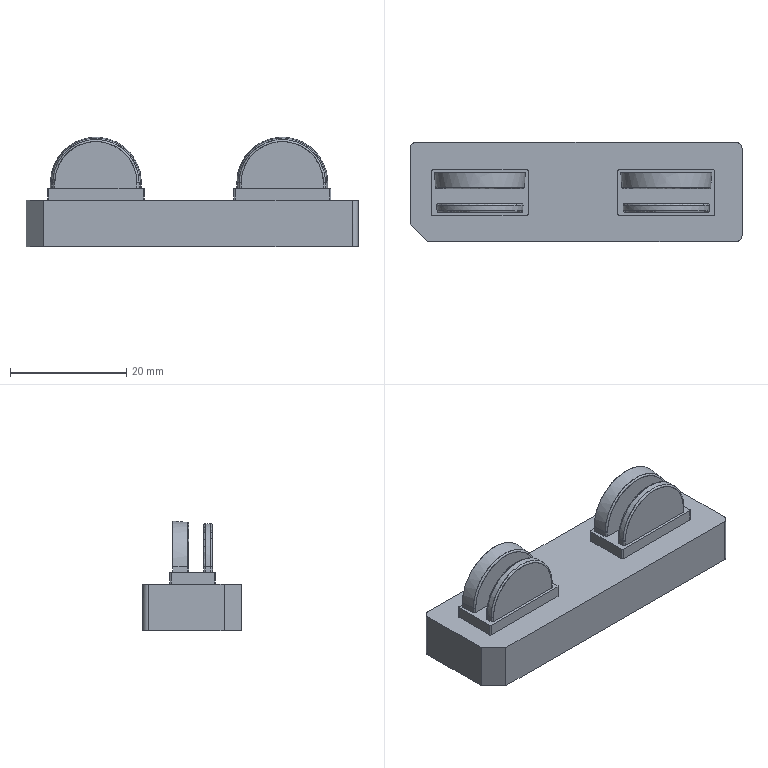NC program | PowerMill | posted by the shop | part box 57 x 17 x 18.807 mm
Lines 16994 to 18566 of 381081:
( TOOL ID   D2C_1_1 )
( TOOL DIA. 2. TIP RAD 0 LENGTH 64.04 )
( Z = -8.98 )
T28 M6
T3
G91 G28 Z0
G0 G90 G54
M08
S18000 M3
X0 Y0 M8
G43 Z9.797 H28
X13.589 Y-1.296
Z.489
G1 Z-.711 F2400
X13.597 Y-1.311 F4000
G3 X13.795 Y-1.381 I.134 J.064
G1 X14.096 Y-1.236
X14.44 Y-1.152
X15.127 Y-1.08
X15.815 Y-1.079
X16.502 Y-1.142
X16.846 Y-1.218
X17.202 Y-1.371
X17.791 Y-.435
X17.786 Y-.419
G3 X17.599 Y-.323 I-.141 J-.045
G1 X17.534 Y-.344
X16.846 Y-.438
X16.159 Y-.455
X14.096 Y-.436
X13.467 Y-.344
X13.381 Y-.315
X12.957 Y-1.424 Z-.811
X12.968 Y-1.437
G3 X13.177 Y-1.448 I.111 J.099
G1 X13.259 Y-1.375
X13.408 Y-1.293
X13.752 Y-1.171
X14.44 Y-1.05
X15.127 Y-1.021
X16.502 Y-1.045
X17.19 Y-1.152
X17.534 Y-1.266
X17.741 Y-1.375
X17.816 Y-1.437
X18.32 Y-.362
X18.314 Y-.346
G3 X18.123 Y-.26 I-.139 J-.053
G1 X17.902 Y-.344
X17.534 Y-.413
X17.19 Y-.444
X16.502 Y-.46
X13.752 Y-.441
X13.096 Y-.344
X12.849 Y-.247
X12.533 Y-1.473 Z-.91
X12.544 Y-1.485
G3 X12.754 Y-1.5 I.112 J.097
G1 X12.898 Y-1.375
X13.408 Y-1.141
X13.752 Y-1.068
X14.44 Y-1.012
X16.159 Y-1.
X16.921 Y-1.031
X17.534 Y-1.126
X17.878 Y-1.258
X18.101 Y-1.375
X18.221 Y-1.471
X18.249 Y-1.505
X18.725 Y-.317
X18.719 Y-.302
G3 X18.525 Y-.22 I-.138 J-.056
G1 X18.219 Y-.344
X17.878 Y-.411
X17.19 Y-.46
X16.51
X16.502
X16.473
X13.752 Y-.458
X13.408 Y-.444
X12.78 Y-.344
X12.475 Y-.215
X12.199 Y-1.484 Z-1.01
X12.21 Y-1.496
G3 X12.42 Y-1.51 I.112 J.098
G1 X12.573 Y-1.375
X12.721 Y-1.282
X13.064 Y-1.136
X13.408 Y-1.061
X14.096 Y-1.
X16.15
X16.159
X16.16
X16.846
X17.368 Y-1.031
X17.878 Y-1.123
X18.221 Y-1.251
X18.43 Y-1.375
X18.565 Y-1.485
X18.582 Y-1.507
X19.03 Y-.275
X19.023 Y-.26
G3 X18.825 Y-.188 I-.135 J-.063
G1 X18.489 Y-.344
X18.221 Y-.406
X17.534 Y-.46
X17.193
X17.192
X17.19
X16.97
X16.505
X16.502
X16.494
X13.408 Y-.459
X13.064 Y-.442
X12.511 Y-.344
X12.171 Y-.179
X11.907 Y-1.562 Z-1.11
X11.919 Y-1.574
G3 X12.129 Y-1.566 I.101 J.109
G1 X12.306 Y-1.375
X12.721 Y-1.152
X13.064 Y-1.058
X13.752 Y-1.
X17.19
X17.878 Y-1.048
X18.221 Y-1.135
X18.695 Y-1.375
X18.888 Y-1.55
X19.316 Y-.232
X19.308 Y-.218
G3 X19.105 Y-.162 I-.129 J-.073
G1 X18.909 Y-.274
X18.73 Y-.344
X18.221 Y-.442
X17.708 Y-.46
X17.193
X17.192
X17.19
X16.97
X16.505
X16.502
X16.494
X13.408 Y-.459
X13.064 Y-.457
X12.721 Y-.438
X12.377 Y-.369
X12.033 Y-.243
X11.898 Y-.159
G0 Z2.991
G1 X19.563 Y-.181 F10000
G0 Z-.009
G1 Z-1.209 F2400
X19.553 Y-.168 F4000
G3 X19.344 Y-.141 I-.118 J-.091
G1 X19.253 Y-.212
X18.965 Y-.344
X18.565 Y-.433
X17.878 Y-.46
X13.064
X12.377 Y-.424
X12.034 Y-.344
X11.689 Y-.176
X11.652 Y-.149
Y-1.551
X11.664 Y-1.562
G3 X11.874 Y-1.553 I.1 J.109
G1 X12.033 Y-1.38
X12.377 Y-1.181
X12.721 Y-1.076
X12.978 Y-1.031
X13.408 Y-1.
X17.534
X18.221 Y-1.061
X18.565 Y-1.159
X18.909 Y-1.342
X19.129 Y-1.556
G0 Z2.891
G1 X11.412 Y-1.581 F10000
G0 Z-.109
G1 Z-1.309 F2400
X11.425 Y-1.591 F4000
G3 X11.634 Y-1.563 I.09 J.118
G1 X11.689 Y-1.491
X12.033 Y-1.232
X12.377 Y-1.098
X12.712 Y-1.031
X13.064 Y-1.
X17.878
X18.221 Y-1.024
X18.565 Y-1.082
X18.909 Y-1.202
X19.253 Y-1.439
X19.373 Y-1.583
X19.785 Y-.204
X19.778 Y-.19
G3 X19.578 Y-.126 I-.132 J-.068
G1 X19.157 Y-.344
X18.909 Y-.411
X18.221 Y-.46
X17.879
X17.878
X13.064
X13.063
X13.062
X12.719
X12.377 Y-.447
X12.033 Y-.395
X11.689 Y-.286
X11.425 Y-.109
G0 Z2.792
G1 X19.985 Y-.163 F10000
G0 Z-.208
G1 Z-1.408 F2400
X19.976 Y-.15 F4000
G3 X19.769 Y-.114 I-.121 J-.086
G1 X19.597 Y-.236
X19.348 Y-.344
X18.909 Y-.441
X18.565 Y-.46
X12.377
X12.033 Y-.435
X11.652 Y-.344
X11.345 Y-.2
X11.231 Y-.117
X11.202 Y-1.589
X11.215 Y-1.6
G3 X11.424 Y-1.591 I.1 J.11
G1 X11.622 Y-1.375
X12.033 Y-1.145
X12.377 Y-1.044
X12.721 Y-1.002
X13.04
X13.064 Y-1.
X17.878
X17.879
X18.221
X18.565 Y-1.036
X18.909 Y-1.123
X19.253 Y-1.28
X19.578 Y-1.563
X20.183 Y-.144 Z-1.508
X20.172 Y-.131
G3 X19.964 Y-.109 I-.116 J-.093
G1 X19.94 Y-.127
X19.539 Y-.344
X19.253 Y-.421
X18.909 Y-.441
X18.76 Y-.449
X18.565 Y-.46
X12.377
X12.033 Y-.451
X11.689 Y-.408
X11.345 Y-.302
X11.038 Y-.093
X11.006 Y-1.581
X11.018 Y-1.592
G3 X11.227 Y-1.572 I.095 J.114
G1 X11.345 Y-1.43
X11.689 Y-1.197
X12.033 Y-1.073
X12.26 Y-1.031
X12.721 Y-1.
X18.221
X18.565 Y-1.008
X18.909 Y-1.058
X19.253 Y-1.173
X19.586 Y-1.375
X19.772 Y-1.583
X20.36 Y-.118 Z-1.608
X20.35 Y-.105
G3 X20.142 Y-.08 I-.117 J-.091
G1 X19.94 Y-.237
X19.696 Y-.344
X19.253 Y-.443
X18.909 Y-.46
X12.033
X11.689 Y-.437
X11.345 Y-.357
X11.002 Y-.199
X10.849 Y-.08
X10.817 Y-1.57
X10.829 Y-1.582
G3 X11.039 Y-1.585 I.107 J.103
G1 X11.345 Y-1.289
X11.689 Y-1.12
X12.033 Y-1.034
X12.377 Y-1.
X12.718
X12.719
X12.721
X18.221
X18.223
X18.565
X18.909 Y-1.026
X19.253 Y-1.098
X19.597 Y-1.251
X19.94 Y-1.547
X19.96 Y-1.575
X20.523 Y-.122 Z-1.707
X20.513 Y-.109
G3 X20.304 Y-.088 I-.115 J-.094
G1 X20.284 Y-.105
X19.94 Y-.314
X19.853 Y-.344
X19.597 Y-.42
X19.253 Y-.456
X18.909 Y-.46
X12.033
X11.689 Y-.452
X11.345 Y-.406
X11.002 Y-.289
X10.705 Y-.081
X10.662 Y-1.593
X10.674 Y-1.604
G3 X10.884 Y-1.584 I.095 J.114
G1 X11.002 Y-1.441
X11.345 Y-1.194
X11.689 Y-1.063
X11.865 Y-1.031
X12.377 Y-1.
X12.568
X12.72
X12.721
X18.221
X18.223
X18.565
X18.587 Y-1.002
X18.909
X19.253 Y-1.051
X19.597 Y-1.171
X19.928 Y-1.375
X20.125 Y-1.6
X20.666 Y-.114 Z-1.807
X20.656 Y-.101
G3 X20.447 Y-.082 I-.114 J-.095
G1 X20.284 Y-.217
X20.009 Y-.344
X19.597 Y-.441
X19.253 Y-.46
X11.689
X11.345 Y-.434
X10.991 Y-.344
X10.658 Y-.175
X10.535 Y-.079
X10.489 Y-1.57
X10.501 Y-1.582
G3 X10.711 Y-1.584 I.106 J.104
G1 X11.002 Y-1.298
X11.345 Y-1.125
X11.689 Y-1.032
X12.033 Y-1.
X18.909
X19.253 Y-1.023
X19.597 Y-1.101
X19.94 Y-1.257
X20.284 Y-1.561
X20.287 Y-1.565
X20.831 Y-.105 Z-1.907
X20.822 Y-.092
G3 X20.615 Y-.058 I-.121 J-.086
G1 X20.284 Y-.294
X20.114 Y-.359
X19.94 Y-.413
X19.597 Y-.456
X19.253 Y-.46
X11.689
X11.345 Y-.45
X11.002 Y-.397
X10.658 Y-.267
X10.381 Y-.058
X10.339 Y-1.605
X10.351 Y-1.615
G3 X10.56 Y-1.596 I.095 J.114
G1 X10.744 Y-1.375
X11.002 Y-1.202
X11.345 Y-1.066
X11.53 Y-1.031
X12.033 Y-1.
X12.252
X18.909
X18.933 Y-1.002
X19.253
X19.597 Y-1.053
X19.94 Y-1.174
X20.256 Y-1.375
X20.445 Y-1.603
X20.98 Y-.085 Z-2.006
X20.969 Y-.073
G3 X20.76 Y-.055 I-.114 J-.096
G1 X20.628 Y-.166
X20.286 Y-.344
X19.94 Y-.436
X19.597 Y-.46
X11.345
X11.002 Y-.429
X10.713 Y-.344
X10.314 Y-.118
X10.248 Y-.062
X10.191 Y-1.618
X10.203 Y-1.628
G3 X10.412 Y-1.609 I.095 J.114
G1 X10.607 Y-1.375
X11.002 Y-1.136
X11.345 Y-1.035
X11.689 Y-1.
X19.253
X19.597 Y-1.025
X19.94 Y-1.11
X20.284 Y-1.287
X20.393 Y-1.375
X20.579 Y-1.599
G0 Z2.596
G1 X10.061 Y-1.608 F10000
G0 Z-.906
G1 Z-2.106 F2400
X10.074 Y-1.617 F4000
G3 X10.281 Y-1.584 I.087 J.12
G1 X10.314 Y-1.539
X10.47 Y-1.375
X10.658 Y-1.238
X11.002 Y-1.081
X11.227 Y-1.031
X11.689 Y-1.
X18.909
X18.93
X19.253
X19.281 Y-1.002
X19.597 Y-1.004
X19.94 Y-1.065
X20.284 Y-1.209
X20.529 Y-1.375
X20.717 Y-1.6
X21.103 Y-.089
X21.093 Y-.076
G3 X20.885 Y-.051 I-.117 J-.092
G1 X20.628 Y-.252
X20.458 Y-.327
X20.284 Y-.392
X19.94 Y-.45
X19.597 Y-.46
X11.345
X11.002 Y-.444
X10.658 Y-.371
X10.314 Y-.217
X10.112 Y-.039
X9.92 Y-1.613 Z-2.205
X9.933 Y-1.624
G3 X10.142 Y-1.604 I.095 J.114
G1 X10.333 Y-1.375
X10.658 Y-1.17
X11.002 Y-1.048
X11.345 Y-1.
X19.597
X19.91 Y-1.031
X20.284 Y-1.142
X20.628 Y-1.342
X20.853 Y-1.603
X21.241 Y-.082
X21.23 Y-.069
G3 X21.021 Y-.055 I-.112 J-.098
G1 X20.972 Y-.098
X20.546 Y-.344
X20.284 Y-.425
X19.94 Y-.459
X19.611
X19.597 Y-.46
X12.394
X11.689
X11.681
X11.345
X11.301 Y-.458
X11.002 Y-.456
X10.658 Y-.412
X10.314 Y-.288
X9.977 Y-.054
X9.799 Y-1.615 Z-2.305
X9.812 Y-1.626
G3 X10.021 Y-1.603 I.093 J.116
G1 X10.204 Y-1.375
X10.314 Y-1.287
X10.658 Y-1.106
X10.953 Y-1.031
X11.345 Y-1.
X19.597
X19.94 Y-1.013
X20.284 Y-1.086
X20.628 Y-1.249
X20.796 Y-1.375
X20.976 Y-1.599
X21.368 Y-.066
X21.357 Y-.054
G3 X21.147 Y-.039 I-.112 J-.097
G1 X20.972 Y-.191
X20.675 Y-.344
X20.284 Y-.441
X19.94 Y-.46
X11.002
X10.658 Y-.434
X10.325 Y-.344
X9.97 Y-.145
X9.853 Y-.04
X9.683 Y-1.619 Z-2.405
X9.695 Y-1.629
G3 X9.904 Y-1.606 I.093 J.116
G1 X10.09 Y-1.375
X10.314 Y-1.219
X10.658 Y-1.066
X11.002 Y-1.003
X11.311
X11.345 Y-1.
X19.597
X19.607
X19.94
X20.182 Y-1.031
X20.628 Y-1.187
X20.91 Y-1.375
X21.101 Y-1.613
X21.475 Y-.068
X21.465 Y-.055
G3 X21.256 Y-.032 I-.116 J-.093
G1 X20.972 Y-.26
X20.802 Y-.336
X20.628 Y-.4
X20.284 Y-.454
X19.94 Y-.46
X11.002
X10.658 Y-.448
X10.314 Y-.382
X9.97 Y-.226
X9.741 Y-.035
X9.562 Y-1.626 Z-2.504
X9.575 Y-1.637
G3 X9.784 Y-1.614 I.093 J.116
G1 X9.976 Y-1.375
X10.314 Y-1.157
X10.658 Y-1.041
X11.002 Y-1.
X19.94
X20.284 Y-1.029
X20.628 Y-1.128
X20.972 Y-1.33
X21.211 Y-1.614
X21.603 Y-.047
X21.592 Y-.035
G3 X21.382 Y-.026 I-.11 J-.1
G1 X21.316 Y-.086
X20.892 Y-.344
X20.628 Y-.426
X20.284 Y-.46
X19.941
X19.94
X11.002
X10.946 Y-.458
X10.658
X10.314 Y-.414
X9.97 Y-.286
X9.628 Y-.035
X9.456 Y-1.617 Z-2.604
X9.469 Y-1.627
G3 X9.678 Y-1.604 I.093 J.116
G1 X9.862 Y-1.375
X9.97 Y-1.288
X10.314 Y-1.104
X10.587 Y-1.031
X11.002 Y-1.
X19.94
X20.284 Y-1.009
X20.628 Y-1.083
X20.972 Y-1.251
X21.138 Y-1.375
X21.317 Y-1.598
X21.699 Y-.061
X21.688 Y-.049
G3 X21.478 Y-.035 I-.112 J-.098
G1 X21.316 Y-.178
X21.001 Y-.344
X20.628 Y-.44
X20.284 Y-.46
X10.658
X10.314 Y-.434
X9.999 Y-.344
X9.626 Y-.131
X9.511 Y-.027
G0 Z2.732
G1 X21.803 Y-.048 F10000
G0 Z-1.504
G1 Z-2.704 F2400
X21.793 Y-.035 F4000
G3 X21.583 Y-.019 I-.113 J-.097
G1 X21.316 Y-.25
X21.146 Y-.329
X20.972 Y-.395
X20.628 Y-.451
X20.284 Y-.46
X10.658
X10.314 Y-.446
X9.97 Y-.376
X9.626 Y-.214
X9.414 Y-.011
X9.347 Y-1.62
X9.36 Y-1.63
G3 X9.568 Y-1.605 I.092 J.117
G1 X9.748 Y-1.375
X9.97 Y-1.219
X10.314 Y-1.066
X10.658 Y-1.003
X10.97 Y-1.002
X11.002 Y-1.
X19.94
X19.943
X20.284
X20.526 Y-1.031
X20.972 Y-1.187
X21.252 Y-1.375
X21.436 Y-1.611
X21.903 Y-.06 Z-2.803
X21.894 Y-.046
G3 X21.686 Y-.017 I-.119 J-.089
G1 X21.316 Y-.296
X21.208 Y-.344
X20.972 Y-.422
X20.628 Y-.46
X10.658
X10.314 Y-.455
X9.97 Y-.408
X9.626 Y-.267
X9.316 Y-.017
X9.236 Y-1.641
X9.249 Y-1.651
G3 X9.457 Y-1.623 I.09 J.118
G1 X9.626 Y-1.401
X9.97 Y-1.161
X10.314 Y-1.043
X10.658 Y-1.
X20.284
X20.628 Y-1.03
X20.972 Y-1.131
X21.316 Y-1.347
X21.539 Y-1.624
G0 Z2.555
G1 X9.138 Y-1.644 F10000
G0 Z-1.703
G1 Z-2.903 F2400
X9.151 Y-1.655 F4000
G3 X9.359 Y-1.629 I.091 J.117
G1 X9.557 Y-1.375
X9.97 Y-1.114
X10.26 Y-1.031
X10.658 Y-1.
X20.284
X20.628 Y-1.011
X20.972 Y-1.092
X21.316 Y-1.275
X21.443 Y-1.375
X21.629 Y-1.614
X22.012 Y-.025
X22.001 Y-.013
G3 X21.791 Y-.008 I-.107 J-.103
G1 X21.659 Y-.134
X21.299 Y-.344
X20.972 Y-.435
X20.628 Y-.46
X15.929
X10.658
X10.654
X10.314
X9.97 Y-.428
X9.701 Y-.344
X9.283 Y-.08
X9.208 Y-.006
X9.05 Y-1.635 Z-3.003
X9.063 Y-1.646
G3 X9.271 Y-1.62 I.091 J.117
G1 X9.462 Y-1.375
X9.626 Y-1.252
X9.97 Y-1.08
X10.314 Y-1.006
X10.742 Y-.999
X11.17 Y-1.
X20.284
X20.314 Y-1.001
X20.628
X20.972 Y-1.063
X21.316 Y-1.217
X21.538 Y-1.375
X21.723 Y-1.612
X22.087 Y-.046
X22.076 Y-.034
G3 X21.867 Y-.021 I-.111 J-.098
G1 X21.659 Y-.205
X21.39 Y-.344
X20.972 Y-.446
X20.628 Y-.46
X10.314
X9.97 Y-.439
X9.626 Y-.351
X9.283 Y-.162
X9.115 Y-.004
X8.957 Y-1.632 Z-3.102
X8.97 Y-1.643
G3 X9.178 Y-1.617 I.091 J.117
G1 X9.366 Y-1.375
X9.626 Y-1.195
X9.97 Y-1.055
X10.314 Y-1.
X10.656
X10.658
X10.971
X20.628
X20.936 Y-1.031
X21.316 Y-1.161
X21.633 Y-1.375
X21.821 Y-1.616
X22.178 Y-.048
X22.167 Y-.035
G3 X21.958 Y-.015 I-.115 J-.094
G1 X21.659 Y-.26
X21.49 Y-.34
X21.316 Y-.405
X20.972 Y-.457
X20.689
X20.628 Y-.46
X10.537
X10.253 Y-.459
X9.97 Y-.451
X9.626 Y-.387
X9.283 Y-.227
X9.034 Y.001
X8.861 Y-1.644 Z-3.202
X8.874 Y-1.654
G3 X9.083 Y-1.627 I.091 J.118
G1 X9.276 Y-1.375
X9.626 Y-1.142
X9.972 Y-1.031
X10.314 Y-1.
X20.628
X20.972 Y-1.019
X21.316 Y-1.115
X21.726 Y-1.375
X21.92 Y-1.63
X22.283 Y.046
X22.269 Y.055
G3 X22.062 Y.02 I-.086 J-.121
G1 X22.003 Y-.064
X21.572 Y-.344
X21.316 Y-.426
X20.972 Y-.46
X18.441
X10.537
X10.314
X10.284 Y-.459
X9.97
X9.626 Y-.414
X9.283 Y-.277
X8.942 Y-.005
X8.783 Y-1.642 Z-3.301
X8.796 Y-1.652
G3 X9.004 Y-1.625 I.09 J.118
G1 X9.196 Y-1.375
X9.283 Y-1.303
X9.626 Y-1.104
X9.882 Y-1.031
X10.314 Y-1.
X20.628
X20.972 Y-1.007
X21.316 Y-1.083
X21.659 Y-1.263
X21.805 Y-1.375
X21.989 Y-1.616
X22.347 Y-.027
X22.335 Y-.015
G3 X22.125 Y-.015 I-.105 J-.105
G1 X22.003 Y-.138
X21.656 Y-.344
X21.316 Y-.437
X20.972 Y-.46
X9.97
X9.626 Y-.43
X9.345 Y-.344
X8.939 Y-.084
X8.859 Y0
X8.856 Y.005
G0 Z2.861
G1 X22.443 Y.016 F10000
G0 Z-2.201
G1 Z-3.401 F2400
X22.43 Y.026 F4000
G3 X22.221 Y.005 I-.094 J-.115
G1 X22.217 Y0
X22.003 Y-.198
X21.732 Y-.344
X21.316 Y-.448
X20.972 Y-.46
X9.97
X9.626 Y-.439
X9.283 Y-.35
X8.939 Y-.153
X8.782 Y0
X8.778 Y.006
X8.707 Y-1.638
X8.72 Y-1.648
G3 X8.928 Y-1.621 I.09 J.118
G1 X9.116 Y-1.375
X9.283 Y-1.249
X9.626 Y-1.077
X9.97 Y-1.003
X10.314 Y-1.
X12.704
X20.628
X20.637
X20.972
X21.316 Y-1.06
X21.659 Y-1.213
X21.884 Y-1.375
X22.077 Y-1.627
X22.497 Y-.029 Z-3.501
X22.486 Y-.016
G3 X22.276 Y-.004 I-.111 J-.099
G1 X22.003 Y-.247
X21.808 Y-.344
X21.659 Y-.4
X21.316 Y-.456
X20.972 Y-.46
X9.97
X9.626 Y-.449
X9.283 Y-.381
X8.939 Y-.21
X8.706 Y0
X8.7 Y.008
X8.623 Y-1.644
X8.636 Y-1.654
G3 X8.844 Y-1.626 I.09 J.118
G1 X9.037 Y-1.375
X9.283 Y-1.199
X9.626 Y-1.055
X9.97 Y-1.
X20.972
X21.285 Y-1.031
X21.659 Y-1.163
X21.964 Y-1.375
X22.154 Y-1.624
G0 Z2.506
G1 X8.538 Y-1.652 F10000
G0 Z-2.4
G1 Z-3.6 F2400
X8.551 Y-1.662 F4000
G3 X8.759 Y-1.632 I.089 J.119
G1 X8.939 Y-1.393
X9.283 Y-1.152
X9.64 Y-1.031
X9.97 Y-1.
X20.972
X21.316 Y-1.022
X21.659 Y-1.123
X22.003 Y-1.341
X22.234 Y-1.629
X22.581 Y-.044
X22.571 Y-.031
G3 X22.363 Y-.005 I-.117 J-.092
G1 X22.003 Y-.287
X21.885 Y-.344
X21.659 Y-.419
X21.316 Y-.46
X20.982
X20.972
X9.97
X9.897 Y-.458
X9.626 Y-.457
X9.283 Y-.406
X8.939 Y-.257
X8.63 Y0
X8.625 Y.008
X8.465 Y-1.666 Z-3.7
X8.479 Y-1.675
G3 X8.686 Y-1.642 I.087 J.12
G1 X8.878 Y-1.375
X9.283 Y-1.114
X9.563 Y-1.031
X9.97 Y-1.
X20.972
X21.316 Y-1.01
X21.659 Y-1.091
X22.003 Y-1.28
X22.122 Y-1.375
X22.31 Y-1.618
X22.671 Y.056
X22.656 Y.065
G3 X22.453 Y.015 I-.077 J-.127
G1 X22.444 Y0
X22.347 Y-.103
X21.961 Y-.344
X21.659 Y-.432
X21.316 Y-.46
X9.626
X9.283 Y-.423
X8.939 Y-.295
X8.595 Y-.043
X8.558 Y.012
G0 Z2.725
G1 X22.745 Y.063 F10000
G0 Z-2.599
G1 Z-3.799 F2400
X22.731 Y.072 F4000
G3 X22.526 Y.029 I-.081 J-.124
G1 X22.507 Y0
X22.347 Y-.159
X22.032 Y-.344
X21.659 Y-.441
X21.316 Y-.46
X9.626
X9.283 Y-.434
X8.968 Y-.344
X8.595 Y-.107
X8.493 Y0
X8.47 Y.035
X8.396 Y-1.654
X8.409 Y-1.664
G3 X8.617 Y-1.635 I.089 J.119
G1 X8.812 Y-1.375
X8.939 Y-1.276
X9.283 Y-1.086
X9.484 Y-1.031
X9.97 Y-1.
X10.377
X20.972
X21.021 Y-1.001
X21.316
X21.659 Y-1.069
X22.003 Y-1.236
X22.188 Y-1.375
X22.383 Y-1.635
X22.808 Y.03 Z-3.899
X22.795 Y.041
G3 X22.586 Y.019 I-.094 J-.115
G1 X22.57 Y0
X22.347 Y-.207
X22.096 Y-.344
X21.659 Y-.451
X21.316 Y-.46
X9.626
X9.283 Y-.444
X8.939 Y-.358
X8.595 Y-.163
X8.429 Y0
X8.417 Y.017
X8.334 Y-1.65
X8.347 Y-1.66
G3 X8.555 Y-1.63 I.089 J.119
G1 X8.746 Y-1.375
X8.939 Y-1.231
X9.283 Y-1.067
X9.626 Y-1.001
X9.958
X9.97 Y-1.
X10.377
X20.246
X21.316
X21.584 Y-1.031
X22.003 Y-1.192
X22.254 Y-1.375
X22.45 Y-1.637
G0 Z2.563
G1 X8.269 Y-1.648 F10000
G0 Z-2.799
G1 Z-3.999 F2400
X8.282 Y-1.658 F4000
G3 X8.49 Y-1.629 I.089 J.119
G1 X8.681 Y-1.375
X8.939 Y-1.187
X9.283 Y-1.048
X9.626 Y-1.
X21.316
X21.659 Y-1.034
X22.003 Y-1.154
X22.32 Y-1.375
X22.519 Y-1.641
X22.867 Y.003
X22.856 Y.015
G3 X22.646 Y.025 I-.11 J-.1
G1 X22.347 Y-.246
X22.159 Y-.344
X22.003 Y-.402
X21.659 Y-.457
X21.403 Y-.458
X21.316 Y-.46
X9.9
X9.591 Y-.459
X9.283 Y-.453
X8.939 Y-.383
X8.595 Y-.209
X8.366 Y0
X8.35 Y.019
X8.191 Y-1.665 Z-4.098
X8.205 Y-1.675
G3 X8.412 Y-1.643 I.088 J.12
G1 X8.595 Y-1.395
X8.939 Y-1.149
X9.278 Y-1.031
X9.626 Y-1.
X21.316
X21.659 Y-1.017
X22.003 Y-1.121
X22.347 Y-1.341
X22.582 Y-1.642
X22.93 Y.055
X22.916 Y.064
G3 X22.711 Y.021 I-.081 J-.124
G1 X22.697 Y0
X22.347 Y-.28
X22.223 Y-.344
X22.003 Y-.418
X21.659 Y-.46
X21.316
X9.9
X9.626
X9.503 Y-.457
X9.283
X8.939 Y-.404
X8.595 Y-.249
X8.303 Y0
X8.283 Y.029
X8.134 Y-1.678 Z-4.198
X8.148 Y-1.687
G3 X8.355 Y-1.651 I.086 J.121
G1 X8.55 Y-1.375
X8.939 Y-1.118
X9.218 Y-1.031
X9.626 Y-1.
X21.316
X21.659 Y-1.009
X22.003 Y-1.095
X22.347 Y-1.291
X22.451 Y-1.375
X22.644 Y-1.627
X22.987 Y.059
X22.973 Y.069
G3 X22.766 Y.032 I-.085 J-.122
G1 X22.691 Y-.076
X22.286 Y-.344
X22.003 Y-.429
X21.659 Y-.46
X9.283
X8.939 Y-.419
X8.595 Y-.282
X8.251 Y-.013
X8.226 Y.025
X8.072 Y-1.661 Z-4.298
X8.085 Y-1.671
G3 X8.293 Y-1.64 I.088 J.119
G1 X8.489 Y-1.375
X8.595 Y-1.29
X8.939 Y-1.092
X9.153 Y-1.031
X9.626 Y-1.
X9.913
X21.316
X21.395 Y-1.002
X21.659
X22.003 Y-1.074
X22.347 Y-1.248
X22.511 Y-1.375
X22.706 Y-1.639
X23.056 Y.066
X23.042 Y.074
G3 X22.837 Y.03 I-.081 J-.125
G1 X22.817 Y0
X22.691 Y-.132
X22.349 Y-.344
X22.003 Y-.438
X21.659 Y-.46
X9.283
X8.939 Y-.429
X8.651 Y-.344
X8.251 Y-.078
X8.158 Y.058
G0 Z2.848
G1 X23.115 Y.055 F10000
G0 Z-3.197
G1 Z-4.397 F2400
X23.101 Y.065 F4000
G3 X22.894 Y.033 I-.088 J-.12
G1 X22.869 Y0
X22.691 Y-.175
X22.401 Y-.344
X22.003 Y-.447
X21.659 Y-.46
X9.283
X8.939 Y-.438
X8.595 Y-.341
X8.251 Y-.126
X8.131 Y0
X8.097 Y.053
X8.017 Y-1.664
X8.03 Y-1.674
G3 X8.238 Y-1.643 I.088 J.119
G1 X8.436 Y-1.375
X8.595 Y-1.251
X8.939 Y-1.074
X9.283 Y-1.002
X9.598
X9.626 Y-1.
X9.913
X21.316
X21.317
X21.659
X21.908 Y-1.031
X22.347 Y-1.21
X22.564 Y-1.375
X22.691 Y-1.519
X22.767 Y-1.638
X23.168 Y.044 Z-4.497
X23.155 Y.055
G3 X22.946 Y.032 I-.093 J-.116
G1 X22.921 Y0
X22.691 Y-.211
X22.453 Y-.344
X22.347 Y-.386
X22.003 Y-.453
X21.659 Y-.46
X9.283
X8.939 Y-.446
X8.595 Y-.365
X8.251 Y-.17
X8.079 Y0
X8.043 Y.05
X7.959 Y-1.677
X7.973 Y-1.686
G3 X8.178 Y-1.64 I.08 J.125
G1 X8.251 Y-1.525
X8.382 Y-1.375
X8.595 Y-1.213
X8.939 Y-1.059
X9.283 Y-1.
X21.659
X21.965 Y-1.031
X22.347 Y-1.176
X22.617 Y-1.375
X22.819 Y-1.646
G0 Z2.489
G1 X7.898 Y-1.685 F10000
G0 Z-3.396
G1 Z-4.596 F2400
X7.911 Y-1.694 F4000
G3 X8.118 Y-1.654 I.083 J.123
G1 X8.251 Y-1.456
X8.595 Y-1.179
X8.939 Y-1.044
X9.283 Y-1.
X21.659
X22.003 Y-1.028
X22.347 Y-1.146
X22.671 Y-1.375
X22.875 Y-1.651
X23.217 Y.016
X23.206 Y.029
G3 X22.996 Y.037 I-.109 J-.101
G1 X22.691 Y-.244
X22.505 Y-.344
X22.347 Y-.403
X22.003 Y-.458
X21.775
X21.659 Y-.46
X9.58
X9.259
X8.939 Y-.453
X8.595 Y-.385
X8.251 Y-.207
X8.027 Y0
X8.002 Y.032
X7.85 Y-1.672 Z-4.696
X7.864 Y-1.682
G3 X8.071 Y-1.649 I.087 J.12
G1 X8.251 Y-1.399
X8.595 Y-1.149
X8.927 Y-1.031
X9.283 Y-1.
X21.659
X22.003 Y-1.017
X22.347 Y-1.121
X22.691 Y-1.345
X22.926 Y-1.65
X23.256 Y.051
X23.242 Y.06
G3 X23.037 Y.015 I-.08 J-.125
G1 X23.035 Y.011
X22.691 Y-.272
X22.557 Y-.344
X22.347 Y-.416
X22.003 Y-.46
X21.363
X9.58
X9.283
X9.161 Y-.457
X8.939
X8.595 Y-.401
X8.251 Y-.241
X7.975 Y0
X7.954 Y.032
X7.801 Y-1.666 Z-4.796
X7.815 Y-1.676
G3 X8.022 Y-1.645 I.088 J.119
G1 X8.222 Y-1.375
X8.595 Y-1.123
X8.876 Y-1.031
X9.283 Y-1.
X21.659
X22.003 Y-1.01
X22.347 Y-1.099
X22.777 Y-1.375
X22.984 Y-1.653
X23.321 Y.075
X23.307 Y.084
G3 X23.102 Y.04 I-.081 J-.125
G1 X23.076 Y0
X22.609 Y-.344
X22.347 Y-.426
X22.003 Y-.46
X8.939
X8.595 Y-.415
X8.251 Y-.27
X7.923 Y0
X7.903 Y.031
X7.747 Y-1.691 Z-4.895
X7.76 Y-1.7
G3 X7.968 Y-1.666 I.086 J.121
G1 X8.175 Y-1.375
X8.595 Y-1.101
X8.825 Y-1.031
X9.283 Y-1.
X9.513
X21.659
X21.76 Y-1.003
X22.003
X22.347 Y-1.081
X22.691 Y-1.268
X22.825 Y-1.375
X23.026 Y-1.639
X23.377 Y.093
X23.363 Y.102
G3 X23.158 Y.056 I-.08 J-.125
G1 X23.122 Y0
X23.035 Y-.097
X22.658 Y-.344
X22.347 Y-.435
X22.003 Y-.46
X8.939
X8.595 Y-.424
X8.341 Y-.344
X7.907 Y-.034
X7.84 Y.069
X7.714 Y-1.668 Z-4.995
X7.727 Y-1.678
G3 X7.935 Y-1.646 I.088 J.12
G1 X8.133 Y-1.375
X8.251 Y-1.28
X8.595 Y-1.087
X8.817 Y-1.034
X8.825 Y-1.031
X8.829
X8.939 Y-1.005
X9.283 Y-1.
X12.606
X21.659
X21.67 Y-1.001
X22.003
X22.347 Y-1.068
X22.691 Y-1.237
X22.867 Y-1.375
X23.065 Y-1.645
X23.415 Y.089
X23.401 Y.098
G3 X23.196 Y.052 I-.08 J-.125
G1 X23.163 Y0
X23.035 Y-.133
X22.7 Y-.344
X22.347 Y-.441
X22.003 Y-.46
X8.939
X8.595 Y-.432
X8.3 Y-.344
X7.907 Y-.08
X7.807 Y.067
G0 Z2.742
G1 X23.443 F10000
G0 Z-3.895
G1 Z-5.095 F2400
X23.429 Y.076 F4000
G3 X23.224 Y.031 I-.08 J-.125
G1 X23.204 Y0
X23.035 Y-.168
X22.741 Y-.344
X22.347 Y-.447
X22.003 Y-.46
X8.939
X8.595 Y-.438
X8.258 Y-.344
X7.907 Y-.119
X7.796 Y0
X7.773 Y.036
X7.676 Y-1.661
X7.69 Y-1.671
G3 X7.897 Y-1.639 I.088 J.12
G1 X8.09 Y-1.375
X8.251 Y-1.249
X8.595 Y-1.074
X8.939 Y-1.001
X9.216
X9.283 Y-1.
X12.606
X19.776
X22.003
X22.263 Y-1.031
X22.691 Y-1.206
X22.91 Y-1.375
X23.035 Y-1.517
X23.11 Y-1.636
X23.491 Y.051 Z-5.194
X23.478 Y.061
G3 X23.27 Y.032 I-.09 J-.118
G1 X23.245 Y0
X23.035 Y-.199
X22.782 Y-.344
X22.347 Y-.453
X22.003 Y-.46
X8.939
X8.595 Y-.445
X8.251 Y-.359
X7.907 Y-.155
X7.755 Y0
X7.72 Y.05
X7.627 Y-1.679
X7.641 Y-1.688
G3 X7.845 Y-1.64 I.078 J.126
G1 X7.907 Y-1.539
X8.048 Y-1.375
X8.251 Y-1.217
X8.595 Y-1.06
X8.939 Y-1.
X22.003
X22.307 Y-1.031
X22.691 Y-1.179
X22.952 Y-1.375
X23.155 Y-1.652
G0 Z2.596
G1 X7.584 Y-1.678 F10000
G0 Z-4.094
G1 Z-5.294 F2400
X7.598 Y-1.687 F4000
G3 X7.803 Y-1.643 I.081 J.125
G1 X7.907 Y-1.482
X8.005 Y-1.375
X8.251 Y-1.189
X8.595 Y-1.047
X8.939 Y-1.
X22.003
X22.347 Y-1.031
X22.691 Y-1.154
X22.995 Y-1.375
X23.195 Y-1.648
X23.532 Y.042
X23.519 Y.053
G3 X23.31 Y.03 I-.093 J-.116
G1 X23.286 Y0
X23.035 Y-.226
X22.823 Y-.344
X22.691 Y-.395
X22.347 Y-.457
X22.116
X22.003 Y-.46
X9.227
X8.911 Y-.459
X8.595 Y-.449
X8.251 Y-.375
X7.907 Y-.187
X7.713 Y0
X7.676 Y.05
X7.535 Y-1.684 Z-5.393
X7.549 Y-1.693
G3 X7.755 Y-1.654 I.084 J.123
G1 X7.907 Y-1.431
X8.251 Y-1.163
X8.595 Y-1.035
X8.939 Y-1.
X22.003
X22.347 Y-1.021
X22.691 Y-1.133
X23.037 Y-1.375
X23.24 Y-1.651
X23.57 Y.013
X23.558 Y.026
G3 X23.349 Y.035 I-.11 J-.1
G1 X23.035 Y-.251
X22.864 Y-.344
X22.691 Y-.408
X22.347 Y-.459
X22.02
X22.003 Y-.46
X11.988
X8.939
X8.595 Y-.453
X8.251 Y-.39
X7.907 Y-.215
X7.672 Y0
X7.635 Y.047
X7.502 Y-1.679 Z-5.493
X7.516 Y-1.689
G3 X7.723 Y-1.654 I.086 J.121
G1 X7.907 Y-1.394
X8.251 Y-1.142
X8.568 Y-1.031
X8.939 Y-1.
X22.003
X22.347 Y-1.015
X22.691 Y-1.115
X23.035 Y-1.341
X23.272 Y-1.651
X23.604 Y.072
X23.59 Y.08
G3 X23.385 Y.034 I-.079 J-.126
G1 X23.364 Y0
X23.035 Y-.272
X22.905 Y-.344
X22.691 Y-.417
X22.347 Y-.46
X9.626
X9.596
X8.939
X8.819 Y-.457
X8.595
X8.251 Y-.402
X7.907 Y-.239
X7.636 Y0
X7.605 Y.049
X7.47 Y-1.678 Z-5.593
X7.484 Y-1.687
G3 X7.691 Y-1.654 I.087 J.12
G1 X7.894 Y-1.375
X8.251 Y-1.127
X8.535 Y-1.031
X8.939 Y-1.
X22.003
X22.347 Y-1.011
X22.691 Y-1.102
X23.106 Y-1.375
X23.315 Y-1.663
X23.654 Y.103
X23.64 Y.112
G3 X23.435 Y.067 I-.08 J-.125
G1 X23.378 Y-.021
X22.936 Y-.344
X22.691 Y-.423
X22.347 Y-.46
X16.857
X9.626
X9.605
X8.595
X8.251 Y-.411
X8.064 Y-.344
X7.907 Y-.257
X7.605 Y0
X7.579 Y.041
X7.436 Y-1.68 Z-5.692
X7.45 Y-1.69
G3 X7.657 Y-1.657 I.087 J.12
G1 X7.862 Y-1.375
X8.251 Y-1.113
X8.503 Y-1.031
X8.939 Y-1.
X22.003
X22.347 Y-1.007
X22.691 Y-1.09
X23.035 Y-1.291
X23.138 Y-1.375
X23.335 Y-1.645
X23.68 Y.1
X23.666 Y.11
G3 X23.461 Y.068 I-.082 J-.124
G1 X23.378 Y-.056
X22.968 Y-.344
X22.691 Y-.428
X22.347 Y-.46
X8.595
X8.251 Y-.419
X8.032 Y-.344
X7.907 Y-.275
X7.573 Y0
X7.548 Y.04
X7.405 Y-1.686 Z-5.792
X7.419 Y-1.696
G3 X7.626 Y-1.661 I.086 J.121
G1 X7.829 Y-1.375
X8.251 Y-1.099
X8.47 Y-1.031
X8.939 Y-1.
X9.215
X22.003
X22.132 Y-1.003
X22.347
X22.691 Y-1.079
X23.035 Y-1.266
X23.171 Y-1.375
X23.369 Y-1.634
X23.713 Y.095
X23.699 Y.104
G3 X23.494 Y.058 I-.079 J-.126
G1 X23.458 Y0
X23.378 Y-.089
X22.999 Y-.344
X22.691 Y-.434
X22.347 Y-.46
X8.595
X8.251 Y-.424
X8.001 Y-.344
X7.564 Y-.025
X7.502 Y.07
X7.384 Y-1.663 Z-5.892
X7.397 Y-1.672
G3 X7.605 Y-1.64 I.087 J.12
G1 X7.797 Y-1.375
X7.907 Y-1.285
X8.251 Y-1.088
X8.41 Y-1.05
X8.451 Y-1.035
X8.494 Y-1.03
X8.595 Y-1.006
X8.939 Y-1.
X11.67
X22.003
X22.024 Y-1.001
X22.347
X22.691 Y-1.069
X23.035 Y-1.241
X23.203 Y-1.375
X23.394 Y-1.638
X23.737 Y.091
X23.723 Y.1
G3 X23.519 Y.049 I-.077 J-.127
G1 X23.489 Y0
X23.378 Y-.118
X23.031 Y-.344
X22.691 Y-.439
X22.347 Y-.46
X8.595
X8.251 Y-.429
X7.969 Y-.344
X7.564 Y-.061
X7.488 Y.051
X7.359 Y-1.653 Z-5.991
X7.372 Y-1.663
G3 X7.579 Y-1.63 I.087 J.12
G1 X7.764 Y-1.375
X7.907 Y-1.259
X8.251 Y-1.077
X8.595 Y-1.002
X8.843
X8.939 Y-1.
X11.67
X20.615
X22.347
X22.597 Y-1.031
X22.684 Y-1.068
X22.691 Y-1.07
X22.71 Y-1.079
X23.035 Y-1.216
X23.236 Y-1.375
X23.378 Y-1.542
X23.429 Y-1.626
X23.755 Y.062
X23.741 Y.071
G3 X23.536 Y.025 I-.079 J-.126
G1 X23.521 Y0
X23.378 Y-.146